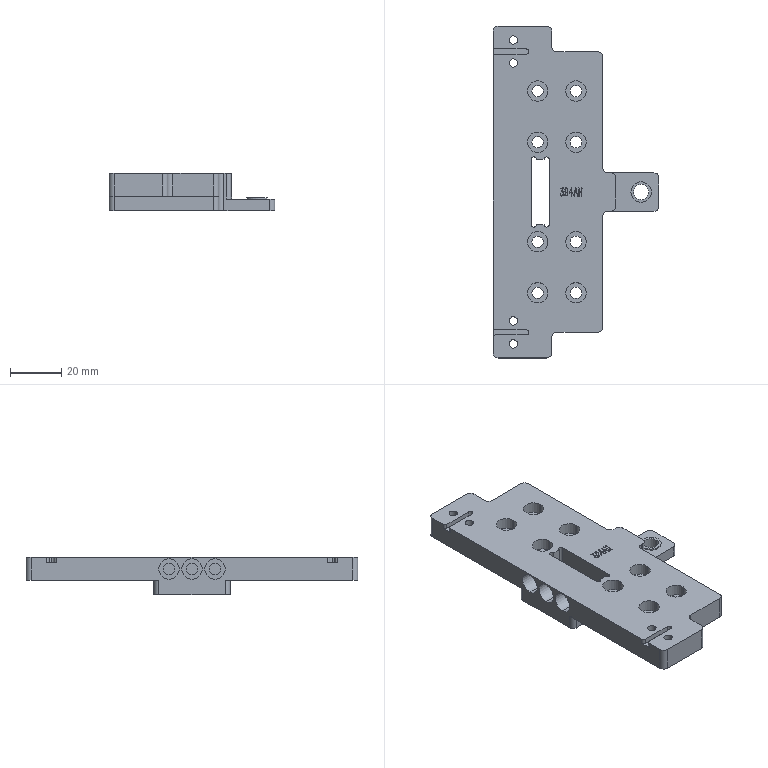NC program | NX | posted with a generic post | part box 65 x 130 x 14.5 mm
Whole program:
N10 G17 G21 G94 G90
(DRILLING_COPY_1_COPY , TOOL : D6A45)
N12 T01 M6
N14 G54
N16 G17 G0 G90 X9. Y-4.5 B0. C0. S5000 M3
N18 G43 Z30. H1
N20 G94 G81 G98 Z-1. F350. R3.
N22 X0.
N24 X-9.
N26 G80
N28 G0 X-9. Y-4.5 Z30.
N30 M5
(DRILLING_COPY_1_COPY_COPY , TOOL : 4.5ZT)
N32 T08 M6
N34 G54
N36 G17 G0 G90 X9. Y-4.5 B0. C0. S2000 M3
N38 G43 Z30. H8
N40 G94 G83 G98 Z-17.852 F200. Q2. R3.
N42 X0.
N44 X-9.
N46 G80
N48 G0 X-9. Y-4.5 Z30.
N50 M5
(HOLE_MILLING_1 , TOOL : D6)
N52 T12 M6
N54 G54
N56 G17 G0 G90 X-9. Y-4.5 B0. C0. S9500 M3
N58 G43 Z30. H12
N60 Z0.5
N62 G94 G3 X-9.5 Y-4. R0.5 F1400.
N64 X-10. Y-4.5 R0.5
N66 X-10. Y-4.5 Z0. I1. J0.
N68 X-10. Y-4.5 Z-0.5 I1. J0.
N70 X-10. Y-4.5 Z-1. I1. J0.
N72 X-10. Y-4.5 Z-1.5 I1. J0.
N74 X-10. Y-4.5 Z-2. I1. J0.
N76 X-10. Y-4.5 Z-2.5 I1. J0.
N78 X-10. Y-4.5 Z-3. I1. J0.
N80 X-10. Y-4.5 Z-3.5 I1. J0.
N82 X-10. Y-4.5 Z-4. I1. J0.
N84 X-10. Y-4.5 Z-4.5 I1. J0.
N86 X-10. Y-4.5 Z-5. I1. J0.
N88 X-10. Y-4.5 Z-5.5 I1. J0.
N90 X-10. Y-4.5 Z-6. I1. J0.
N92 X-10. Y-4.5 Z-6.5 I1. J0.
N94 X-10. Y-4.5 Z-7. I1. J0.
N96 X-10. Y-4.5 Z-7.5 I1. J0.
N98 X-10. Y-4.5 Z-8. I1. J0.
N100 X-10. Y-4.5 Z-8.5 I1. J0.
N102 X-9. Y-5.5 R1.
N104 X-10. Y-4.5 R-1.
N106 X-9.5 Y-5. R0.5
N108 X-9. Y-4.5 R0.5
N110 G0 Z30.
N112 X0.
N114 Z0.5
N116 G3 X-0.5 Y-4. R0.5
N118 X-1. Y-4.5 R0.5
N120 X-1. Y-4.5 Z0. I1. J0.
N122 X-1. Y-4.5 Z-0.5 I1. J0.
N124 X-1. Y-4.5 Z-1. I1. J0.
N126 X-1. Y-4.5 Z-1.5 I1. J0.
N128 X-1. Y-4.5 Z-2. I1. J0.
N130 X-1. Y-4.5 Z-2.5 I1. J0.
N132 X-1. Y-4.5 Z-3. I1. J0.
N134 X-1. Y-4.5 Z-3.5 I1. J0.
N136 X-1. Y-4.5 Z-4. I1. J0.
N138 X-1. Y-4.5 Z-4.5 I1. J0.
N140 X-1. Y-4.5 Z-5. I1. J0.
N142 X-1. Y-4.5 Z-5.5 I1. J0.
N144 X-1. Y-4.5 Z-6. I1. J0.
N146 X-1. Y-4.5 Z-6.5 I1. J0.
N148 X-1. Y-4.5 Z-7. I1. J0.
N150 X-1. Y-4.5 Z-7.5 I1. J0.
N152 X-1. Y-4.5 Z-8. I1. J0.
N154 X-1. Y-4.5 Z-8.5 I1. J0.
N156 X0. Y-5.5 R1.
N158 X-1. Y-4.5 R-1.
N160 X-0.5 Y-5. R0.5
N162 X0. Y-4.5 R0.5
N164 G0 Z30.
N166 X9.
N168 Z0.5
N170 G3 X8.5 Y-4. R0.5
N172 X8. Y-4.5 R0.5
N174 X8. Y-4.5 Z0. I1. J0.
N176 X8. Y-4.5 Z-0.5 I1. J0.
N178 X8. Y-4.5 Z-1. I1. J0.
N180 X8. Y-4.5 Z-1.5 I1. J0.
N182 X8. Y-4.5 Z-2. I1. J0.
N184 X8. Y-4.5 Z-2.5 I1. J0.
N186 X8. Y-4.5 Z-3. I1. J0.
N188 X8. Y-4.5 Z-3.5 I1. J0.
N190 X8. Y-4.5 Z-4. I1. J0.
N192 X8. Y-4.5 Z-4.5 I1. J0.
N194 X8. Y-4.5 Z-5. I1. J0.
N196 X8. Y-4.5 Z-5.5 I1. J0.
N198 X8. Y-4.5 Z-6. I1. J0.
N200 X8. Y-4.5 Z-6.5 I1. J0.
N202 X8. Y-4.5 Z-7. I1. J0.
N204 X8. Y-4.5 Z-7.5 I1. J0.
N206 X8. Y-4.5 Z-8. I1. J0.
N208 X8. Y-4.5 Z-8.5 I1. J0.
N210 X9. Y-5.5 R1.
N212 X8. Y-4.5 R-1.
N214 X8.5 Y-5. R0.5
N216 X9. Y-4.5 R0.5
N218 G0 Z30.
N220 M5
(PLANAR_MILL_COPY_COPY_COPY_COPY_COPY_COPY_1_COPY_COPY_1 , TOOL : D6A45)
N222 T01 M6
N224 G54
N226 G17 G0 G90 X9.6 Y-2.697 B0. C0. S9500 M3
N228 G43 Z30. H1
N230 Z0.5
N232 G94 G1 Z-1. F1250.
N234 X9.866 Y-1.9
N236 G3 X9. Y-1.4 R1.
N238 X5.9 Y-4.5 R3.1
N240 X9. Y-1.4 R-3.1
N242 X8.134 Y-1.9 R1.
N244 G1 X8.4 Y-2.697
N246 Z0.5
N248 G0 Z30.
N250 X0.6
N252 Z0.5
N254 G1 Z-1.
N256 X0.866 Y-1.9
N258 G3 X0. Y-1.4 R1.
N260 X-3.1 Y-4.5 R3.1
N262 X0. Y-1.4 R-3.1
N264 X-0.866 Y-1.9 R1.
N266 G1 X-0.6 Y-2.697
N268 Z0.5
N270 G0 Z30.
N272 X-8.4
N274 Z0.5
N276 G1 Z-1.
N278 X-8.134 Y-1.9
N280 G3 X-9. Y-1.4 R1.
N282 X-12.1 Y-4.5 R3.1
N284 X-9. Y-1.4 R-3.1
N286 X-9.866 Y-1.9 R1.
N288 G1 X-9.6 Y-2.697
N290 Z0.5
N292 G0 Z30.
N294 M5
N296 M2